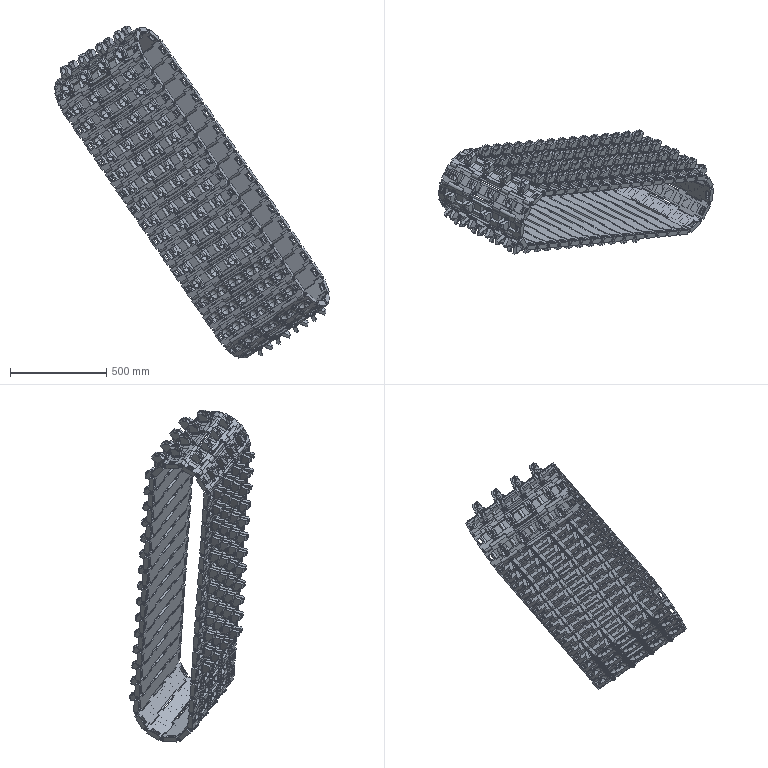Part | SolidWorks | 1216 solids | 28576 faces | volume 41212392 mm3 | plane 13072 | cylinder 10336 | cone 3800 | torus 760 | sphere 608 | commonest cylinder face diameters 3 x3648 10 x2964 20 x1976 8 x608 12 x608 50 x304